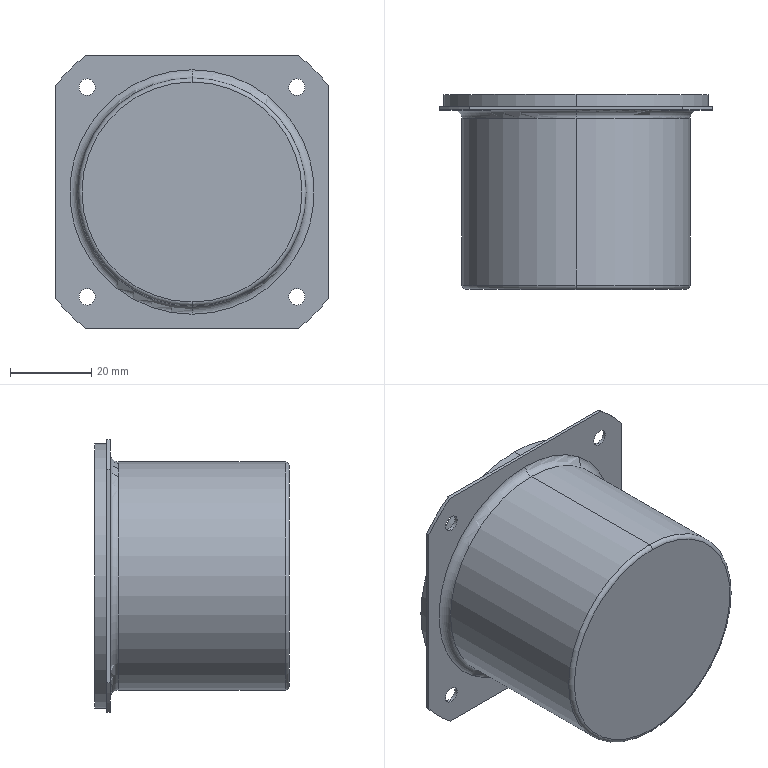Part | STEP file | Speaker 001 | 1 solid | 31 faces | box 67 x 47.8 x 67 mm | volume 121623 mm3 | cylinder 18 | plane 9 | torus 4 | commonest cylinder face diameters 4 x8 85 x4 56 x2 61 x2 65 x2